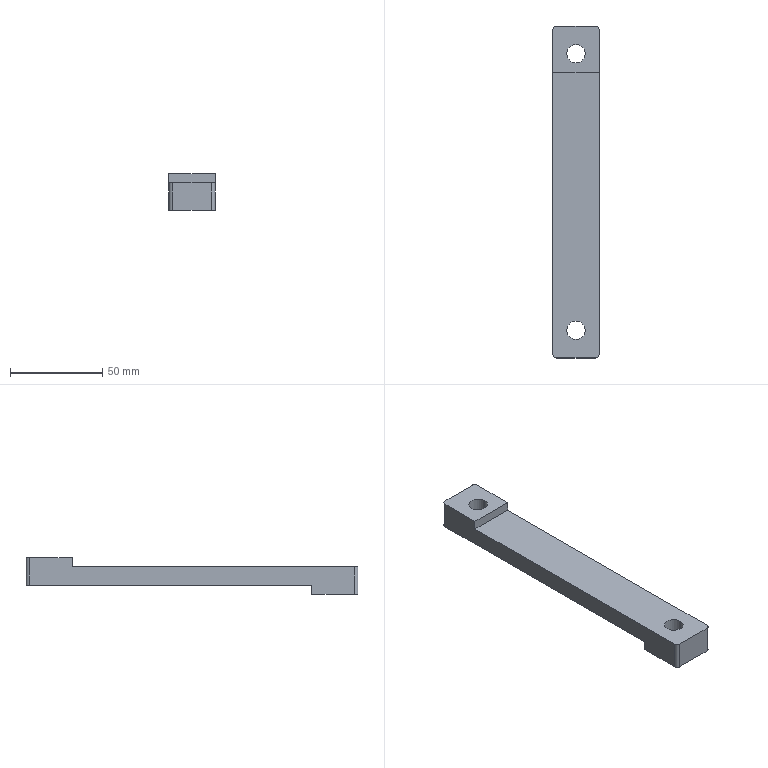Part | SolidWorks | 1 solid | 18 faces | box 25 x 180 x 20 mm | volume 48842 mm3 | plane 10 | cylinder 8 | commonest cylinder face diameters 4 x4 10 x4
STEP:
#1=CARTESIAN_POINT('',(-5.,75.,-5.));
#2=VERTEX_POINT('',#1);
#3=CARTESIAN_POINT('',(5.,75.,-5.));
#4=VERTEX_POINT('',#3);
#5=CARTESIAN_POINT('',(0.,75.,-5.));
#6=DIRECTION('',(0.,0.,1.));
#7=DIRECTION('',(1.,0.,0.));
#8=AXIS2_PLACEMENT_3D('',#5,#6,#7);
#9=CIRCLE('',#8,5.);
#10=EDGE_CURVE('',#2,#4,#9,.T.);
#11=ORIENTED_EDGE('',*,*,#10,.F.);
#12=CARTESIAN_POINT('',(-5.,75.,10.));
#13=VERTEX_POINT('',#12);
#14=CARTESIAN_POINT('',(-5.,75.,-5.));
#15=DIRECTION('',(0.,0.,1.));
#16=VECTOR('',#15,1000.);
#17=LINE('',#14,#16);
#18=EDGE_CURVE('',#2,#13,#17,.T.);
#19=ORIENTED_EDGE('',*,*,#18,.T.);
#20=CARTESIAN_POINT('',(5.,75.,10.));
#21=VERTEX_POINT('',#20);
#22=CARTESIAN_POINT('',(0.,75.,10.));
#23=DIRECTION('',(0.,0.,1.));
#24=DIRECTION('',(1.,0.,0.));
#25=AXIS2_PLACEMENT_3D('',#22,#23,#24);
#26=CIRCLE('',#25,5.);
#27=EDGE_CURVE('',#13,#21,#26,.T.);
#28=ORIENTED_EDGE('',*,*,#27,.T.);
#29=CARTESIAN_POINT('',(5.,75.,-5.));
#30=DIRECTION('',(0.,0.,1.));
#31=VECTOR('',#30,1000.);
#32=LINE('',#29,#31);
#33=EDGE_CURVE('',#4,#21,#32,.T.);
#34=ORIENTED_EDGE('',*,*,#33,.F.);
#35=EDGE_LOOP('',(#11,#19,#28,#34));
#36=FACE_OUTER_BOUND('',#35,.T.);
#37=CARTESIAN_POINT('',(0.,75.,-5.));
#38=DIRECTION('',(0.,0.,1.));
#39=DIRECTION('',(1.,0.,0.));
#40=AXIS2_PLACEMENT_3D('',#37,#38,#39);
#41=CYLINDRICAL_SURFACE('',#40,5.);
#42=ADVANCED_FACE('',(#36),#41,.F.);
#43=CARTESIAN_POINT('',(-5.,-75.,5.));
#44=VERTEX_POINT('',#43);
#45=CARTESIAN_POINT('',(5.,-75.,5.));
#46=VERTEX_POINT('',#45);
#47=CARTESIAN_POINT('',(0.,-75.,5.));
#48=DIRECTION('',(0.,0.,1.));
#49=DIRECTION('',(1.,0.,0.));
#50=AXIS2_PLACEMENT_3D('',#47,#48,#49);
#51=CIRCLE('',#50,5.);
#52=EDGE_CURVE('',#44,#46,#51,.T.);
#53=ORIENTED_EDGE('',*,*,#52,.T.);
#54=CARTESIAN_POINT('',(5.,-75.,-10.));
#55=VERTEX_POINT('',#54);
#56=CARTESIAN_POINT('',(5.,-75.,20.));
#57=DIRECTION('',(0.,0.,-1.));
#58=VECTOR('',#57,1000.);
#59=LINE('',#56,#58);
#60=EDGE_CURVE('',#46,#55,#59,.T.);
#61=ORIENTED_EDGE('',*,*,#60,.T.);
#62=CARTESIAN_POINT('',(-5.,-75.,-10.));
#63=VERTEX_POINT('',#62);
#64=CARTESIAN_POINT('',(0.,-75.,-10.));
#65=DIRECTION('',(0.,0.,-1.));
#66=DIRECTION('',(-1.,0.,0.));
#67=AXIS2_PLACEMENT_3D('',#64,#65,#66);
#68=CIRCLE('',#67,5.);
#69=EDGE_CURVE('',#55,#63,#68,.T.);
#70=ORIENTED_EDGE('',*,*,#69,.T.);
#71=CARTESIAN_POINT('',(-5.,-75.,20.));
#72=DIRECTION('',(0.,0.,-1.));
#73=VECTOR('',#72,1000.);
#74=LINE('',#71,#73);
#75=EDGE_CURVE('',#44,#63,#74,.T.);
#76=ORIENTED_EDGE('',*,*,#75,.F.);
#77=EDGE_LOOP('',(#53,#61,#70,#76));
#78=FACE_OUTER_BOUND('',#77,.T.);
#79=CARTESIAN_POINT('',(0.,-75.,20.));
#80=DIRECTION('',(0.,0.,-1.));
#81=DIRECTION('',(-1.,0.,0.));
#82=AXIS2_PLACEMENT_3D('',#79,#80,#81);
#83=CYLINDRICAL_SURFACE('',#82,5.);
#84=ADVANCED_FACE('',(#78),#83,.F.);
#85=CARTESIAN_POINT('',(0.,75.,-5.));
#86=DIRECTION('',(0.,0.,1.));
#87=DIRECTION('',(1.,0.,0.));
#88=AXIS2_PLACEMENT_3D('',#85,#86,#87);
#89=CIRCLE('',#88,5.);
#90=EDGE_CURVE('',#4,#2,#89,.T.);
#91=ORIENTED_EDGE('',*,*,#90,.T.);
#92=ORIENTED_EDGE('',*,*,#10,.T.);
#93=EDGE_LOOP('',(#91,#92));
#94=FACE_BOUND('',#93,.T.);
#95=CARTESIAN_POINT('',(-12.5,88.,-5.));
#96=VERTEX_POINT('',#95);
#97=CARTESIAN_POINT('',(-12.5,-65.,-5.));
#98=VERTEX_POINT('',#97);
#99=CARTESIAN_POINT('',(-12.5,90.,-5.));
#100=DIRECTION('',(0.,-1.,0.));
#101=VECTOR('',#100,1000.);
#102=LINE('',#99,#101);
#103=EDGE_CURVE('',#96,#98,#102,.T.);
#104=ORIENTED_EDGE('',*,*,#103,.F.);
#105=CARTESIAN_POINT('',(-10.5,90.,-5.));
#106=VERTEX_POINT('',#105);
#107=CARTESIAN_POINT('',(-10.5,88.,-5.));
#108=DIRECTION('',(0.,0.,-1.));
#109=DIRECTION('',(1.,0.,0.));
#110=AXIS2_PLACEMENT_3D('',#107,#108,#109);
#111=CIRCLE('',#110,2.);
#112=EDGE_CURVE('',#96,#106,#111,.T.);
#113=ORIENTED_EDGE('',*,*,#112,.T.);
#114=CARTESIAN_POINT('',(10.5,90.,-5.));
#115=VERTEX_POINT('',#114);
#116=CARTESIAN_POINT('',(-12.5,90.,-5.));
#117=DIRECTION('',(-1.,0.,0.));
#118=VECTOR('',#117,1000.);
#119=LINE('',#116,#118);
#120=EDGE_CURVE('',#115,#106,#119,.T.);
#121=ORIENTED_EDGE('',*,*,#120,.F.);
#122=CARTESIAN_POINT('',(12.5,88.,-5.));
#123=VERTEX_POINT('',#122);
#124=CARTESIAN_POINT('',(10.5,88.,-5.));
#125=DIRECTION('',(0.,0.,-1.));
#126=DIRECTION('',(1.,0.,0.));
#127=AXIS2_PLACEMENT_3D('',#124,#125,#126);
#128=CIRCLE('',#127,2.);
#129=EDGE_CURVE('',#115,#123,#128,.T.);
#130=ORIENTED_EDGE('',*,*,#129,.T.);
#131=CARTESIAN_POINT('',(12.5,-65.,-5.));
#132=VERTEX_POINT('',#131);
#133=CARTESIAN_POINT('',(12.5,90.,-5.));
#134=DIRECTION('',(0.,1.,0.));
#135=VECTOR('',#134,1000.);
#136=LINE('',#133,#135);
#137=EDGE_CURVE('',#132,#123,#136,.T.);
#138=ORIENTED_EDGE('',*,*,#137,.F.);
#139=CARTESIAN_POINT('',(12.5,-65.,-5.));
#140=DIRECTION('',(1.,0.,0.));
#141=VECTOR('',#140,1000.);
#142=LINE('',#139,#141);
#143=EDGE_CURVE('',#98,#132,#142,.T.);
#144=ORIENTED_EDGE('',*,*,#143,.F.);
#145=EDGE_LOOP('',(#104,#113,#121,#130,#138,#144));
#146=FACE_OUTER_BOUND('',#145,.T.);
#147=CARTESIAN_POINT('',(0.,0.,-5.));
#148=DIRECTION('',(0.,0.,1.));
#149=DIRECTION('',(1.,0.,0.));
#150=AXIS2_PLACEMENT_3D('',#147,#148,#149);
#151=PLANE('',#150);
#152=ADVANCED_FACE('',(#94,#146),#151,.F.);
#153=CARTESIAN_POINT('',(12.5,-88.,5.));
#154=VERTEX_POINT('',#153);
#155=CARTESIAN_POINT('',(12.5,65.,5.));
#156=VERTEX_POINT('',#155);
#157=CARTESIAN_POINT('',(12.5,90.,5.));
#158=DIRECTION('',(0.,1.,0.));
#159=VECTOR('',#158,1000.);
#160=LINE('',#157,#159);
#161=EDGE_CURVE('',#154,#156,#160,.T.);
#162=ORIENTED_EDGE('',*,*,#161,.F.);
#163=CARTESIAN_POINT('',(12.5,-88.,-10.));
#164=VERTEX_POINT('',#163);
#165=CARTESIAN_POINT('',(12.5,-88.,5.));
#166=DIRECTION('',(0.,0.,-1.));
#167=VECTOR('',#166,1000.);
#168=LINE('',#165,#167);
#169=EDGE_CURVE('',#154,#164,#168,.T.);
#170=ORIENTED_EDGE('',*,*,#169,.T.);
#171=CARTESIAN_POINT('',(12.5,-65.,-10.));
#172=VERTEX_POINT('',#171);
#173=CARTESIAN_POINT('',(12.5,-90.,-10.));
#174=DIRECTION('',(0.,-1.,0.));
#175=VECTOR('',#174,1000.);
#176=LINE('',#173,#175);
#177=EDGE_CURVE('',#172,#164,#176,.T.);
#178=ORIENTED_EDGE('',*,*,#177,.F.);
#179=CARTESIAN_POINT('',(12.5,-65.,-10.));
#180=DIRECTION('',(0.,0.,1.));
#181=VECTOR('',#180,1000.);
#182=LINE('',#179,#181);
#183=EDGE_CURVE('',#172,#132,#182,.T.);
#184=ORIENTED_EDGE('',*,*,#183,.T.);
#185=ORIENTED_EDGE('',*,*,#137,.T.);
#186=CARTESIAN_POINT('',(12.5,88.,10.));
#187=VERTEX_POINT('',#186);
#188=CARTESIAN_POINT('',(12.5,88.,5.));
#189=DIRECTION('',(0.,0.,1.));
#190=VECTOR('',#189,1000.);
#191=LINE('',#188,#190);
#192=EDGE_CURVE('',#123,#187,#191,.T.);
#193=ORIENTED_EDGE('',*,*,#192,.T.);
#194=CARTESIAN_POINT('',(12.5,65.,10.));
#195=VERTEX_POINT('',#194);
#196=CARTESIAN_POINT('',(12.5,90.,10.));
#197=DIRECTION('',(0.,1.,0.));
#198=VECTOR('',#197,1000.);
#199=LINE('',#196,#198);
#200=EDGE_CURVE('',#195,#187,#199,.T.);
#201=ORIENTED_EDGE('',*,*,#200,.F.);
#202=CARTESIAN_POINT('',(12.5,65.,10.));
#203=DIRECTION('',(0.,0.,-1.));
#204=VECTOR('',#203,1000.);
#205=LINE('',#202,#204);
#206=EDGE_CURVE('',#195,#156,#205,.T.);
#207=ORIENTED_EDGE('',*,*,#206,.T.);
#208=EDGE_LOOP('',(#162,#170,#178,#184,#185,#193,#201,#207));
#209=FACE_OUTER_BOUND('',#208,.T.);
#210=CARTESIAN_POINT('',(12.5,90.,5.));
#211=DIRECTION('',(-1.,0.,0.));
#212=DIRECTION('',(0.,-1.,0.));
#213=AXIS2_PLACEMENT_3D('',#210,#211,#212);
#214=PLANE('',#213);
#215=ADVANCED_FACE('',(#209),#214,.F.);
#216=ORIENTED_EDGE('',*,*,#120,.T.);
#217=CARTESIAN_POINT('',(-10.5,90.,10.));
#218=VERTEX_POINT('',#217);
#219=CARTESIAN_POINT('',(-10.5,90.,5.));
#220=DIRECTION('',(0.,0.,1.));
#221=VECTOR('',#220,1000.);
#222=LINE('',#219,#221);
#223=EDGE_CURVE('',#106,#218,#222,.T.);
#224=ORIENTED_EDGE('',*,*,#223,.T.);
#225=CARTESIAN_POINT('',(10.5,90.,10.));
#226=VERTEX_POINT('',#225);
#227=CARTESIAN_POINT('',(-12.5,90.,10.));
#228=DIRECTION('',(-1.,0.,0.));
#229=VECTOR('',#228,1000.);
#230=LINE('',#227,#229);
#231=EDGE_CURVE('',#226,#218,#230,.T.);
#232=ORIENTED_EDGE('',*,*,#231,.F.);
#233=CARTESIAN_POINT('',(10.5,90.,5.));
#234=DIRECTION('',(0.,0.,-1.));
#235=VECTOR('',#234,1000.);
#236=LINE('',#233,#235);
#237=EDGE_CURVE('',#226,#115,#236,.T.);
#238=ORIENTED_EDGE('',*,*,#237,.T.);
#239=EDGE_LOOP('',(#216,#224,#232,#238));
#240=FACE_OUTER_BOUND('',#239,.T.);
#241=CARTESIAN_POINT('',(-12.5,90.,5.));
#242=DIRECTION('',(0.,-1.,0.));
#243=DIRECTION('',(0.,0.,-1.));
#244=AXIS2_PLACEMENT_3D('',#241,#242,#243);
#245=PLANE('',#244);
#246=ADVANCED_FACE('',(#240),#245,.F.);
#247=CARTESIAN_POINT('',(-12.5,-88.,-10.));
#248=VERTEX_POINT('',#247);
#249=CARTESIAN_POINT('',(-12.5,-65.,-10.));
#250=VERTEX_POINT('',#249);
#251=CARTESIAN_POINT('',(-12.5,-90.,-10.));
#252=DIRECTION('',(0.,1.,0.));
#253=VECTOR('',#252,1000.);
#254=LINE('',#251,#253);
#255=EDGE_CURVE('',#248,#250,#254,.T.);
#256=ORIENTED_EDGE('',*,*,#255,.F.);
#257=CARTESIAN_POINT('',(-12.5,-88.,5.));
#258=VERTEX_POINT('',#257);
#259=CARTESIAN_POINT('',(-12.5,-88.,5.));
#260=DIRECTION('',(0.,0.,1.));
#261=VECTOR('',#260,1000.);
#262=LINE('',#259,#261);
#263=EDGE_CURVE('',#248,#258,#262,.T.);
#264=ORIENTED_EDGE('',*,*,#263,.T.);
#265=CARTESIAN_POINT('',(-12.5,65.,5.));
#266=VERTEX_POINT('',#265);
#267=CARTESIAN_POINT('',(-12.5,90.,5.));
#268=DIRECTION('',(0.,-1.,0.));
#269=VECTOR('',#268,1000.);
#270=LINE('',#267,#269);
#271=EDGE_CURVE('',#266,#258,#270,.T.);
#272=ORIENTED_EDGE('',*,*,#271,.F.);
#273=CARTESIAN_POINT('',(-12.5,65.,10.));
#274=VERTEX_POINT('',#273);
#275=CARTESIAN_POINT('',(-12.5,65.,10.));
#276=DIRECTION('',(0.,0.,-1.));
#277=VECTOR('',#276,1000.);
#278=LINE('',#275,#277);
#279=EDGE_CURVE('',#274,#266,#278,.T.);
#280=ORIENTED_EDGE('',*,*,#279,.F.);
#281=CARTESIAN_POINT('',(-12.5,88.,10.));
#282=VERTEX_POINT('',#281);
#283=CARTESIAN_POINT('',(-12.5,90.,10.));
#284=DIRECTION('',(0.,-1.,0.));
#285=VECTOR('',#284,1000.);
#286=LINE('',#283,#285);
#287=EDGE_CURVE('',#282,#274,#286,.T.);
#288=ORIENTED_EDGE('',*,*,#287,.F.);
#289=CARTESIAN_POINT('',(-12.5,88.,5.));
#290=DIRECTION('',(0.,0.,-1.));
#291=VECTOR('',#290,1000.);
#292=LINE('',#289,#291);
#293=EDGE_CURVE('',#282,#96,#292,.T.);
#294=ORIENTED_EDGE('',*,*,#293,.T.);
#295=ORIENTED_EDGE('',*,*,#103,.T.);
#296=CARTESIAN_POINT('',(-12.5,-65.,-10.));
#297=DIRECTION('',(0.,0.,1.));
#298=VECTOR('',#297,1000.);
#299=LINE('',#296,#298);
#300=EDGE_CURVE('',#250,#98,#299,.T.);
#301=ORIENTED_EDGE('',*,*,#300,.F.);
#302=EDGE_LOOP('',(#256,#264,#272,#280,#288,#294,#295,#301));
#303=FACE_OUTER_BOUND('',#302,.T.);
#304=CARTESIAN_POINT('',(-12.5,90.,5.));
#305=DIRECTION('',(1.,0.,0.));
#306=DIRECTION('',(0.,1.,0.));
#307=AXIS2_PLACEMENT_3D('',#304,#305,#306);
#308=PLANE('',#307);
#309=ADVANCED_FACE('',(#303),#308,.F.);
#310=CARTESIAN_POINT('',(10.5,-90.,-10.));
#311=VERTEX_POINT('',#310);
#312=CARTESIAN_POINT('',(-10.5,-90.,-10.));
#313=VERTEX_POINT('',#312);
#314=CARTESIAN_POINT('',(12.5,-90.,-10.));
#315=DIRECTION('',(-1.,0.,0.));
#316=VECTOR('',#315,1000.);
#317=LINE('',#314,#316);
#318=EDGE_CURVE('',#311,#313,#317,.T.);
#319=ORIENTED_EDGE('',*,*,#318,.F.);
#320=CARTESIAN_POINT('',(10.5,-90.,5.));
#321=VERTEX_POINT('',#320);
#322=CARTESIAN_POINT('',(10.5,-90.,5.));
#323=DIRECTION('',(0.,0.,1.));
#324=VECTOR('',#323,1000.);
#325=LINE('',#322,#324);
#326=EDGE_CURVE('',#311,#321,#325,.T.);
#327=ORIENTED_EDGE('',*,*,#326,.T.);
#328=CARTESIAN_POINT('',(-10.5,-90.,5.));
#329=VERTEX_POINT('',#328);
#330=CARTESIAN_POINT('',(-12.5,-90.,5.));
#331=DIRECTION('',(1.,0.,0.));
#332=VECTOR('',#331,1000.);
#333=LINE('',#330,#332);
#334=EDGE_CURVE('',#329,#321,#333,.T.);
#335=ORIENTED_EDGE('',*,*,#334,.F.);
#336=CARTESIAN_POINT('',(-10.5,-90.,5.));
#337=DIRECTION('',(0.,0.,-1.));
#338=VECTOR('',#337,1000.);
#339=LINE('',#336,#338);
#340=EDGE_CURVE('',#329,#313,#339,.T.);
#341=ORIENTED_EDGE('',*,*,#340,.T.);
#342=EDGE_LOOP('',(#319,#327,#335,#341));
#343=FACE_OUTER_BOUND('',#342,.T.);
#344=CARTESIAN_POINT('',(-12.5,-90.,5.));
#345=DIRECTION('',(0.,1.,0.));
#346=DIRECTION('',(0.,0.,1.));
#347=AXIS2_PLACEMENT_3D('',#344,#345,#346);
#348=PLANE('',#347);
#349=ADVANCED_FACE('',(#343),#348,.F.);
#350=ORIENTED_EDGE('',*,*,#52,.F.);
#351=CARTESIAN_POINT('',(0.,-75.,5.));
#352=DIRECTION('',(0.,0.,1.));
#353=DIRECTION('',(1.,0.,0.));
#354=AXIS2_PLACEMENT_3D('',#351,#352,#353);
#355=CIRCLE('',#354,5.);
#356=EDGE_CURVE('',#46,#44,#355,.T.);
#357=ORIENTED_EDGE('',*,*,#356,.F.);
#358=EDGE_LOOP('',(#350,#357));
#359=FACE_BOUND('',#358,.T.);
#360=ORIENTED_EDGE('',*,*,#334,.T.);
#361=CARTESIAN_POINT('',(10.5,-88.,5.));
#362=DIRECTION('',(0.,0.,1.));
#363=DIRECTION('',(1.,0.,0.));
#364=AXIS2_PLACEMENT_3D('',#361,#362,#363);
#365=CIRCLE('',#364,2.);
#366=EDGE_CURVE('',#321,#154,#365,.T.);
#367=ORIENTED_EDGE('',*,*,#366,.T.);
#368=ORIENTED_EDGE('',*,*,#161,.T.);
#369=CARTESIAN_POINT('',(-12.5,65.,5.));
#370=DIRECTION('',(1.,0.,0.));
#371=VECTOR('',#370,1000.);
#372=LINE('',#369,#371);
#373=EDGE_CURVE('',#266,#156,#372,.T.);
#374=ORIENTED_EDGE('',*,*,#373,.F.);
#375=ORIENTED_EDGE('',*,*,#271,.T.);
#376=CARTESIAN_POINT('',(-10.5,-88.,5.));
#377=DIRECTION('',(0.,0.,1.));
#378=DIRECTION('',(1.,0.,0.));
#379=AXIS2_PLACEMENT_3D('',#376,#377,#378);
#380=CIRCLE('',#379,2.);
#381=EDGE_CURVE('',#258,#329,#380,.T.);
#382=ORIENTED_EDGE('',*,*,#381,.T.);
#383=EDGE_LOOP('',(#360,#367,#368,#374,#375,#382));
#384=FACE_OUTER_BOUND('',#383,.T.);
#385=CARTESIAN_POINT('',(0.,0.,5.));
#386=DIRECTION('',(0.,0.,1.));
#387=DIRECTION('',(1.,0.,0.));
#388=AXIS2_PLACEMENT_3D('',#385,#386,#387);
#389=PLANE('',#388);
#390=ADVANCED_FACE('',(#359,#384),#389,.T.);
#391=ORIENTED_EDGE('',*,*,#373,.T.);
#392=ORIENTED_EDGE('',*,*,#206,.F.);
#393=CARTESIAN_POINT('',(-12.5,65.,10.));
#394=DIRECTION('',(1.,0.,0.));
#395=VECTOR('',#394,1000.);
#396=LINE('',#393,#395);
#397=EDGE_CURVE('',#274,#195,#396,.T.);
#398=ORIENTED_EDGE('',*,*,#397,.F.);
#399=ORIENTED_EDGE('',*,*,#279,.T.);
#400=EDGE_LOOP('',(#391,#392,#398,#399));
#401=FACE_OUTER_BOUND('',#400,.T.);
#402=CARTESIAN_POINT('',(-12.5,65.,10.));
#403=DIRECTION('',(0.,1.,0.));
#404=DIRECTION('',(0.,0.,1.));
#405=AXIS2_PLACEMENT_3D('',#402,#403,#404);
#406=PLANE('',#405);
#407=ADVANCED_FACE('',(#401),#406,.F.);
#408=CARTESIAN_POINT('',(0.,75.,10.));
#409=DIRECTION('',(0.,0.,1.));
#410=DIRECTION('',(1.,0.,0.));
#411=AXIS2_PLACEMENT_3D('',#408,#409,#410);
#412=CIRCLE('',#411,5.);
#413=EDGE_CURVE('',#21,#13,#412,.T.);
#414=ORIENTED_EDGE('',*,*,#413,.F.);
#415=ORIENTED_EDGE('',*,*,#27,.F.);
#416=EDGE_LOOP('',(#414,#415));
#417=FACE_BOUND('',#416,.T.);
#418=ORIENTED_EDGE('',*,*,#231,.T.);
#419=CARTESIAN_POINT('',(-10.5,88.,10.));
#420=DIRECTION('',(0.,0.,1.));
#421=DIRECTION('',(1.,0.,0.));
#422=AXIS2_PLACEMENT_3D('',#419,#420,#421);
#423=CIRCLE('',#422,2.);
#424=EDGE_CURVE('',#218,#282,#423,.T.);
#425=ORIENTED_EDGE('',*,*,#424,.T.);
#426=ORIENTED_EDGE('',*,*,#287,.T.);
#427=ORIENTED_EDGE('',*,*,#397,.T.);
#428=ORIENTED_EDGE('',*,*,#200,.T.);
#429=CARTESIAN_POINT('',(10.5,88.,10.));
#430=DIRECTION('',(0.,0.,1.));
#431=DIRECTION('',(1.,0.,0.));
#432=AXIS2_PLACEMENT_3D('',#429,#430,#431);
#433=CIRCLE('',#432,2.);
#434=EDGE_CURVE('',#187,#226,#433,.T.);
#435=ORIENTED_EDGE('',*,*,#434,.T.);
#436=EDGE_LOOP('',(#418,#425,#426,#427,#428,#435));
#437=FACE_OUTER_BOUND('',#436,.T.);
#438=CARTESIAN_POINT('',(0.,0.,10.));
#439=DIRECTION('',(0.,0.,1.));
#440=DIRECTION('',(1.,0.,0.));
#441=AXIS2_PLACEMENT_3D('',#438,#439,#440);
#442=PLANE('',#441);
#443=ADVANCED_FACE('',(#417,#437),#442,.T.);
#444=ORIENTED_EDGE('',*,*,#143,.T.);
#445=ORIENTED_EDGE('',*,*,#183,.F.);
#446=CARTESIAN_POINT('',(12.5,-65.,-10.));
#447=DIRECTION('',(1.,0.,0.));
#448=VECTOR('',#447,1000.);
#449=LINE('',#446,#448);
#450=EDGE_CURVE('',#250,#172,#449,.T.);
#451=ORIENTED_EDGE('',*,*,#450,.F.);
#452=ORIENTED_EDGE('',*,*,#300,.T.);
#453=EDGE_LOOP('',(#444,#445,#451,#452));
#454=FACE_OUTER_BOUND('',#453,.T.);
#455=CARTESIAN_POINT('',(12.5,-65.,-10.));
#456=DIRECTION('',(0.,-1.,0.));
#457=DIRECTION('',(0.,0.,-1.));
#458=AXIS2_PLACEMENT_3D('',#455,#456,#457);
#459=PLANE('',#458);
#460=ADVANCED_FACE('',(#454),#459,.F.);
#461=CARTESIAN_POINT('',(0.,-75.,-10.));
#462=DIRECTION('',(0.,0.,-1.));
#463=DIRECTION('',(-1.,0.,0.));
#464=AXIS2_PLACEMENT_3D('',#461,#462,#463);
#465=CIRCLE('',#464,5.);
#466=EDGE_CURVE('',#63,#55,#465,.T.);
#467=ORIENTED_EDGE('',*,*,#466,.F.);
#468=ORIENTED_EDGE('',*,*,#69,.F.);
#469=EDGE_LOOP('',(#467,#468));
#470=FACE_BOUND('',#469,.T.);
#471=ORIENTED_EDGE('',*,*,#177,.T.);
#472=CARTESIAN_POINT('',(10.5,-88.,-10.));
#473=DIRECTION('',(0.,0.,-1.));
#474=DIRECTION('',(1.,0.,0.));
#475=AXIS2_PLACEMENT_3D('',#472,#473,#474);
#476=CIRCLE('',#475,2.);
#477=EDGE_CURVE('',#164,#311,#476,.T.);
#478=ORIENTED_EDGE('',*,*,#477,.T.);
#479=ORIENTED_EDGE('',*,*,#318,.T.);
#480=CARTESIAN_POINT('',(-10.5,-88.,-10.));
#481=DIRECTION('',(0.,0.,-1.));
#482=DIRECTION('',(1.,0.,0.));
#483=AXIS2_PLACEMENT_3D('',#480,#481,#482);
#484=CIRCLE('',#483,2.);
#485=EDGE_CURVE('',#313,#248,#484,.T.);
#486=ORIENTED_EDGE('',*,*,#485,.T.);
#487=ORIENTED_EDGE('',*,*,#255,.T.);
#488=ORIENTED_EDGE('',*,*,#450,.T.);
#489=EDGE_LOOP('',(#471,#478,#479,#486,#487,#488));
#490=FACE_OUTER_BOUND('',#489,.T.);
#491=CARTESIAN_POINT('',(0.,0.,-10.));
#492=DIRECTION('',(0.,0.,1.));
#493=DIRECTION('',(1.,0.,0.));
#494=AXIS2_PLACEMENT_3D('',#491,#492,#493);
#495=PLANE('',#494);
#496=ADVANCED_FACE('',(#470,#490),#495,.F.);
#497=ORIENTED_EDGE('',*,*,#366,.F.);
#498=ORIENTED_EDGE('',*,*,#326,.F.);
#499=ORIENTED_EDGE('',*,*,#477,.F.);
#500=ORIENTED_EDGE('',*,*,#169,.F.);
#501=EDGE_LOOP('',(#497,#498,#499,#500));
#502=FACE_OUTER_BOUND('',#501,.T.);
#503=CARTESIAN_POINT('',(10.5,-88.,5.));
#504=DIRECTION('',(0.,0.,-1.));
#505=DIRECTION('',(-1.,0.,0.));
#506=AXIS2_PLACEMENT_3D('',#503,#504,#505);
#507=CYLINDRICAL_SURFACE('',#506,2.);
#508=ADVANCED_FACE('',(#502),#507,.T.);
#509=ORIENTED_EDGE('',*,*,#381,.F.);
#510=ORIENTED_EDGE('',*,*,#263,.F.);
#511=ORIENTED_EDGE('',*,*,#485,.F.);
#512=ORIENTED_EDGE('',*,*,#340,.F.);
#513=EDGE_LOOP('',(#509,#510,#511,#512));
#514=FACE_OUTER_BOUND('',#513,.T.);
#515=CARTESIAN_POINT('',(-10.5,-88.,5.));
#516=DIRECTION('',(0.,0.,-1.));
#517=DIRECTION('',(-1.,0.,0.));
#518=AXIS2_PLACEMENT_3D('',#515,#516,#517);
#519=CYLINDRICAL_SURFACE('',#518,2.);
#520=ADVANCED_FACE('',(#514),#519,.T.);
#521=ORIENTED_EDGE('',*,*,#424,.F.);
#522=ORIENTED_EDGE('',*,*,#223,.F.);
#523=ORIENTED_EDGE('',*,*,#112,.F.);
#524=ORIENTED_EDGE('',*,*,#293,.F.);
#525=EDGE_LOOP('',(#521,#522,#523,#524));
#526=FACE_OUTER_BOUND('',#525,.T.);
#527=CARTESIAN_POINT('',(-10.5,88.,5.));
#528=DIRECTION('',(0.,0.,-1.));
#529=DIRECTION('',(-1.,0.,0.));
#530=AXIS2_PLACEMENT_3D('',#527,#528,#529);
#531=CYLINDRICAL_SURFACE('',#530,2.);
#532=ADVANCED_FACE('',(#526),#531,.T.);
#533=ORIENTED_EDGE('',*,*,#434,.F.);
#534=ORIENTED_EDGE('',*,*,#192,.F.);
#535=ORIENTED_EDGE('',*,*,#129,.F.);
#536=ORIENTED_EDGE('',*,*,#237,.F.);
#537=EDGE_LOOP('',(#533,#534,#535,#536));
#538=FACE_OUTER_BOUND('',#537,.T.);
#539=CARTESIAN_POINT('',(10.5,88.,5.));
#540=DIRECTION('',(0.,0.,-1.));
#541=DIRECTION('',(-1.,0.,0.));
#542=AXIS2_PLACEMENT_3D('',#539,#540,#541);
#543=CYLINDRICAL_SURFACE('',#542,2.);
#544=ADVANCED_FACE('',(#538),#543,.T.);
#545=ORIENTED_EDGE('',*,*,#60,.F.);
#546=ORIENTED_EDGE('',*,*,#356,.T.);
#547=ORIENTED_EDGE('',*,*,#75,.T.);
#548=ORIENTED_EDGE('',*,*,#466,.T.);
#549=EDGE_LOOP('',(#545,#546,#547,#548));
#550=FACE_OUTER_BOUND('',#549,.T.);
#551=CARTESIAN_POINT('',(0.,-75.,20.));
#552=DIRECTION('',(0.,0.,-1.));
#553=DIRECTION('',(-1.,0.,0.));
#554=AXIS2_PLACEMENT_3D('',#551,#552,#553);
#555=CYLINDRICAL_SURFACE('',#554,5.);
#556=ADVANCED_FACE('',(#550),#555,.F.);
#557=ORIENTED_EDGE('',*,*,#18,.F.);
#558=ORIENTED_EDGE('',*,*,#90,.F.);
#559=ORIENTED_EDGE('',*,*,#33,.T.);
#560=ORIENTED_EDGE('',*,*,#413,.T.);
#561=EDGE_LOOP('',(#557,#558,#559,#560));
#562=FACE_OUTER_BOUND('',#561,.T.);
#563=CARTESIAN_POINT('',(0.,75.,-5.));
#564=DIRECTION('',(0.,0.,1.));
#565=DIRECTION('',(1.,0.,0.));
#566=AXIS2_PLACEMENT_3D('',#563,#564,#565);
#567=CYLINDRICAL_SURFACE('',#566,5.);
#568=ADVANCED_FACE('',(#562),#567,.F.);
#569=CLOSED_SHELL('',(#42,#84,#152,#215,#246,#309,#349,#390,#407,#443,#460,#496,#508,#520,#532,#544,#556,#568));
#570=MANIFOLD_SOLID_BREP('',#569);
#571=CARTESIAN_POINT('',(0.,0.,0.));
#572=DIRECTION('',(0.,0.,1.));
#573=DIRECTION('',(1.,0.,0.));
#574=AXIS2_PLACEMENT_3D('',#571,#572,#573);
#575=(LENGTH_UNIT()NAMED_UNIT(*)SI_UNIT(.MILLI.,.METRE.));
#576=UNCERTAINTY_MEASURE_WITH_UNIT(LENGTH_MEASURE(0.00001),#575,'','');
#577=(NAMED_UNIT(*)PLANE_ANGLE_UNIT()SI_UNIT($,.RADIAN.));
#578=(NAMED_UNIT(*)SI_UNIT($,.STERADIAN.)SOLID_ANGLE_UNIT());
#579=(GEOMETRIC_REPRESENTATION_CONTEXT(3)GLOBAL_UNCERTAINTY_ASSIGNED_CONTEXT((#576))GLOBAL_UNIT_ASSIGNED_CONTEXT((#575,#577,#578))REPRESENTATION_CONTEXT('',''));
#580=ADVANCED_BREP_SHAPE_REPRESENTATION('',(#570,#574),#579);